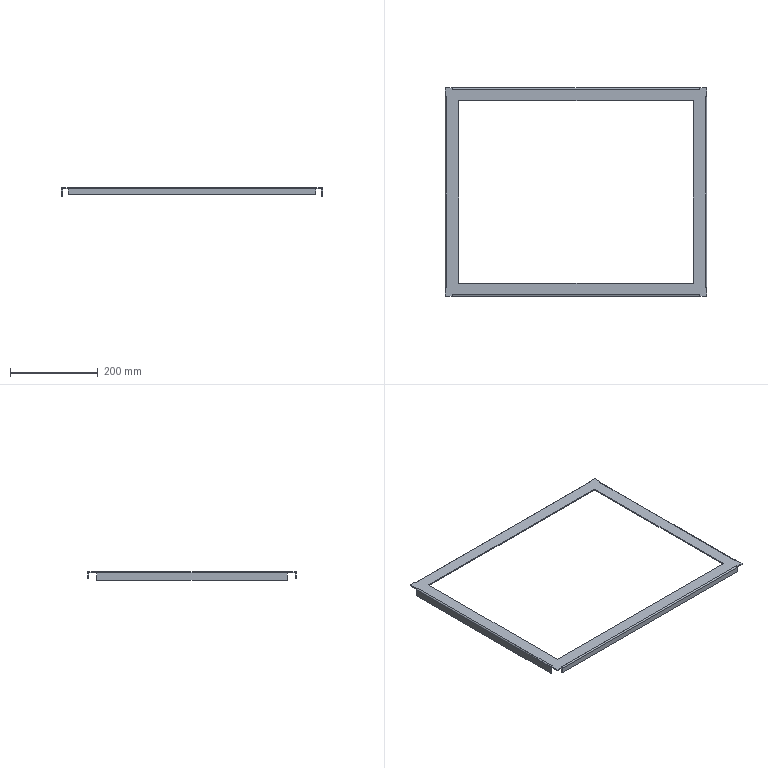Part | SolidWorks | features EdgeFlange 2, MirrorPattern 2, FlatPattern 1, ICE 1, SMBaseFlange 1, SheetMetal 1 | 1 solid | 64 faces | box 596 x 476 x 20 mm | volume 220905 mm3 | plane 56 | cylinder 8 | commonest cylinder face diameters 1 x4 6 x4